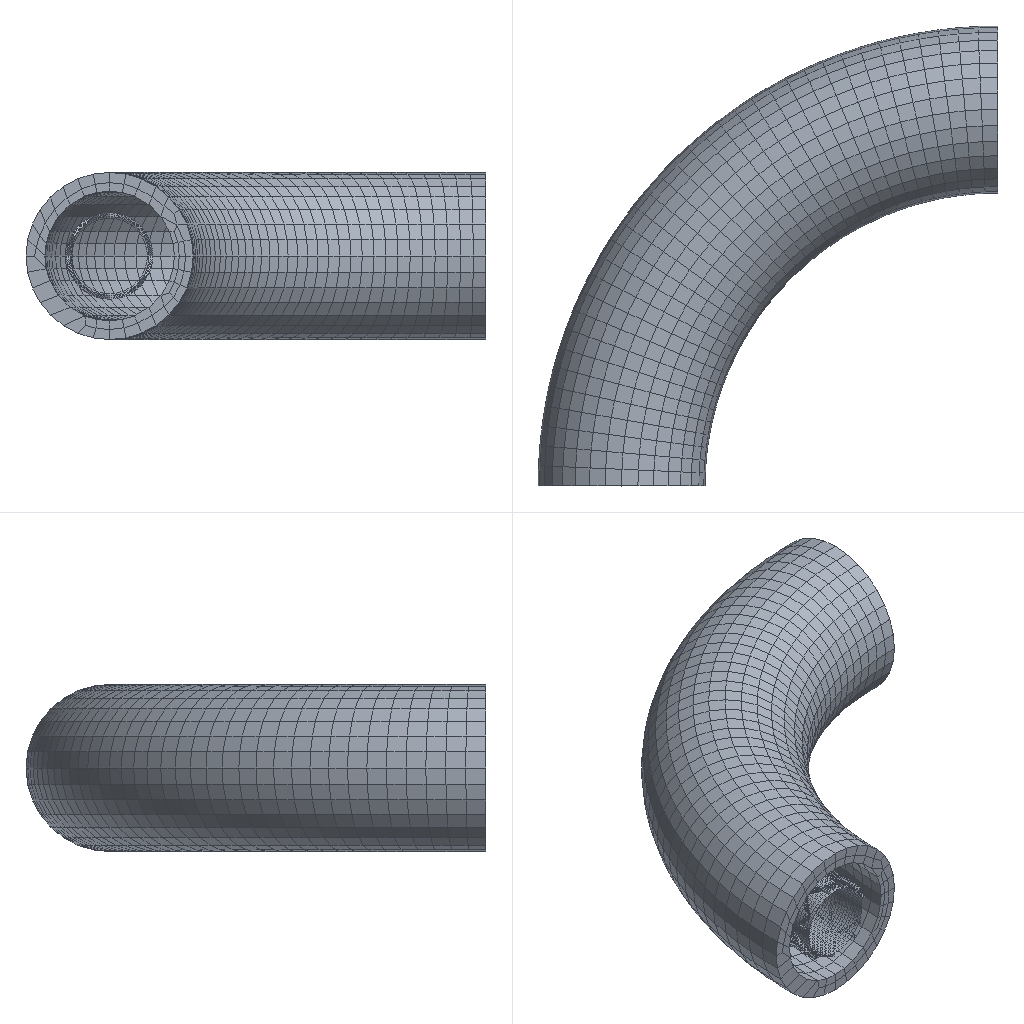Simulation study | abaqus
Set-up summary:
category,name,step,type,value,unit,region
solver,abaqus
solver,version,,,Abaqus/Explicit 2020
units,not stated in the deck,,not stated
analysis,deck,,transient,transient
load_step,Step-1,Step-1,transient
load_step,requested,,,1
mesh,nodes,,,9006
mesh,elements,,,15441
element_type,S4R,,shell,1134
element_type,C3D4H,,solid,12039
element_type,C3D8R,,solid,2268
load,load commands in deck,,count,1
bc,support commands in deck,,count,3
material,SHELL-BALLOON,,in results
material,SS316LN,,in results
material,OGDEN ARTERIAL VESSEL,,in results
check,setup vs results,,match,"per instance, exact: element labels, types and connectivity; labels of the nodes the elements use; coordinates of those nodes at SINGLE_PRECISION in 3 of 3 instance(s)"
Abaqus input file, long lists of numbers shortened:
*Heading
** Job name: Job-2 Model name: Model-1-Copy
** Generated by: Abaqus/CAE 2020
*Preprint, echo=NO, model=NO, history=NO, contact=NO
**
** PARTS
**
*Part, name=P05vessel-r10-220518
*Node
      1,  -12.22,           0., -2.5200424e-09
      2,  -12.177,           0.,  0.4331
** (3439 more lines like these left out)
*Element, type=C3D8R
   1,   68,   66,    1,    2,  161,  159,   94,   95
   2,   34,   66,   68,   33,  127,  159,  161,  126
** (2266 more lines like these left out)
*Nset, nset=Set-1, generate
    1,  3441,     1
*Elset, elset=Set-1, generate
    1,  2268,     1
** Section: Section-2
*Solid Section, elset=Set-1, material="ogden arterial vessel"
,
*End Part
**
*Part, name=Part-1
*Node
      1,  0.995,  0.9, -0.09957
      2,  0.9802,  0.9,  -0.1981
** (1195 more lines like these left out)
*Element, type=S4R
   1,   63,    1,   64,  126
   2,    1,    2,   65,   64
** (1132 more lines like these left out)
*Nset, nset=Set-1, generate
    1,  1197,     1
*Elset, elset=Set-1, generate
    1,  1134,     1
*Nset, nset=Set-3, generate
    1,  1197,     1
*Elset, elset=Set-3, generate
    1,  1134,     1
** Section: Section-1
*Shell Section, elset=Set-1, material=shell-balloon
1., 5
*End Part
**
*Part, name=wrap3layers-R10-220518
*Node
      1, -0.523,  0.55, -0.9058
      2, -0.2032,  0.2828,  -1.026
** (4366 more lines like these left out)
*Element, type=C3D4H
    1, 3584, 3585, 3569, 1457
    2, 3584, 3586,  188, 2546
** (12037 more lines like these left out)
*Nset, nset=Set-1, generate
    1,  4368,     1
*Elset, elset=Set-1, generate
     1,  12039,      1
*Nset, nset=Set-6, generate
    1,  4368,     1
*Elset, elset=Set-6, generate
     1,  12039,      1
** Section: Section-3
*Solid Section, elset=Set-1, material=SS316LN
,
*End Part
**
**
** ASSEMBLY
**
*Assembly, name=Assembly
**
*Instance, name=P05vessel-r10-220518-1, part=P05vessel-r10-220518
   10.11,         -0.9,    -0.284
*End Instance
**
*Instance, name=Part-1-1, part=Part-1
    0.1102,           0.,    -0.284
*End Instance
**
*Instance, name=wrap3layers-R10-220518-1, part=wrap3layers-R10-220518
    0.1102,         -0.9,    -0.284
*End Instance
**
*Nset, nset=Set-1, instance=P05vessel-r10-220518-1, generate
 3349,  3441,     1
*Elset, elset=Set-1, instance=P05vessel-r10-220518-1, generate
 2206,  2268,     1
*Nset, nset=Set-2, instance=Part-1-1, generate
 1135,  1197,     1
*Elset, elset=Set-2, instance=Part-1-1, generate
 1072,  1134,     1
*Nset, nset=Set-3, instance=P05vessel-r10-220518-1, generate
 3349,  3441,     1
*Elset, elset=Set-3, instance=P05vessel-r10-220518-1, generate
 2206,  2268,     1
*Nset, nset=Set-4, instance=Part-1-1, generate
 1135,  1197,     1
*Elset, elset=Set-4, instance=Part-1-1, generate
 1072,  1134,     1
*Nset, nset=Set-5, instance=wrap3layers-R10-220518-1
  135,  136,  137,  138, 1179, 1185
*Elset, elset=Set-5, instance=wrap3layers-R10-220518-1
  2910,  2912, 10089, 10115
*Nset, nset=Set-6, instance=P05vessel-r10-220518-1, generate
  1,  93,   1
*Elset, elset=Set-6, instance=P05vessel-r10-220518-1, generate
  1,  63,   1
*Nset, nset=Set-7, instance=P05vessel-r10-220518-1, generate
  1,  93,   1
*Nset, nset=Set-7, instance=Part-1-1, generate
 1135,  1197,     1
*Elset, elset=Set-7, instance=P05vessel-r10-220518-1, generate
  1,  63,   1
*Elset, elset=Set-7, instance=Part-1-1, generate
 1072,  1134,     1
*Nset, nset=Set-8, instance=P05vessel-r10-220518-1, generate
  1,  93,   1
*Elset, elset=Set-8, instance=P05vessel-r10-220518-1, generate
  1,  63,   1
*Nset, nset=Set-9, instance=Part-1-1, generate
 1135,  1197,     1
*Elset, elset=Set-9, instance=Part-1-1, generate
 1072,  1134,     1
*Nset, nset=Set-10, instance=wrap3layers-R10-220518-1
  135,  136,  137,  138,  147,  148,  149,  150,  159,  160,  161,  162,  287,  288,  289,  290
  299,  300,  301,  302, 1179, 1185, 1244, 1249, 1305, 1309, 2129, 2133, 2192, 2197
*Elset, elset=Set-10, instance=wrap3layers-R10-220518-1
   937,  2442,  2548,  2807,  2910,  2912,  2915,  2916,  4317,  4613,  4618,  4622,  4624,  9087,  9090,  9126
  9561,  9600, 10089, 10115
*Elset, elset=_Surf-7_SPOS, internal, instance=Part-1-1, generate
    1,  1134,     1
*Surface, type=ELEMENT, name=Surf-7
_Surf-7_SPOS, SPOS
*Elset, elset=_Surf-8_SPOS, internal, instance=Part-1-1, generate
    1,  1134,     1
*Surface, type=ELEMENT, name=Surf-8
_Surf-8_SPOS, SPOS
*Elset, elset=_Surf-15_SPOS, internal, instance=Part-1-1, generate
    1,  1134,     1
*Surface, type=ELEMENT, name=Surf-15
_Surf-15_SPOS, SPOS
*Elset, elset=_m_Surf-1_SNEG, internal, instance=Part-1-1, generate
    1,  1134,     1
*Surface, type=ELEMENT, name=m_Surf-1
_m_Surf-1_SNEG, SNEG
*Elset, elset=_m_Surf-3_S3, internal, instance=wrap3layers-R10-220518-1
    50,    60,    77,   128,   131,   135,   347,   433,   439,   440,   470,   475,   486,   493,   502,   539
   718,   754,   759,   775,   972,   979,  1011,  1036,  1055,  1083,  1146,  1174,  1237,  1257,  1259,  1315
** (23 more lines like these left out)
*Elset, elset=_m_Surf-3_S1, internal, instance=wrap3layers-R10-220518-1
   284,  5570,  5738,  6653,  7904,  8010,  8072,  8078,  8127,  8131,  8229,  8243,  8525,  8528,  8577,  8584
  8589,  8590,  8594,  8686,  8801,  9018,  9062,  9678,  9724,  9747,  9774,  9791,  9890, 10009, 10609, 10626
** (1 more lines like these left out)
*Elset, elset=_m_Surf-3_S2, internal, instance=wrap3layers-R10-220518-1
  5035,  5699,  5848,  6144,  6166,  6635,  6637,  6676,  6775,  7137,  7143,  7630,  7856,  8003,  8027,  8079
  8312,  8323,  8374,  8539,  8569,  8587,  8682,  8785,  8803,  8981,  8995,  9064,  9143,  9195,  9200,  9247
** (3 more lines like these left out)
*Elset, elset=_m_Surf-3_S4, internal, instance=wrap3layers-R10-220518-1
  5723,  6031,  6055,  6210,  6217,  6370,  6627,  6659,  6682,  7078,  7167,  7181,  7324,  7532,  7582,  7647
  7669,  7969,  8069,  8073,  8088,  8123,  8258,  8298,  8317,  8322,  8330,  8358,  8526,  8601,  8667,  8672
** (5 more lines like these left out)
*Surface, type=ELEMENT, name=m_Surf-3
_m_Surf-3_S3, S3
_m_Surf-3_S1, S1
_m_Surf-3_S2, S2
_m_Surf-3_S4, S4
*Elset, elset=_m_Surf-5_S3, internal, instance=wrap3layers-R10-220518-1
     5,    50,    60,    69,    77,    91,    95,   108,   110,   115,   128,   131,   135,   144,   169,   207
   213,   329,   347,   372,   415,   433,   439,   440,   450,   453,   470,   475,   486,   493,   502,   539
** (49 more lines like these left out)
*Elset, elset=_m_Surf-5_S1, internal, instance=wrap3layers-R10-220518-1
   174,   284,  1690,  3280,  3431,  3438,  3617,  3763,  3976,  3978,  3998,  4007,  4254,  4260,  4271,  4445
  4488,  4647,  4697,  4716,  4773,  4794,  4946,  5128,  5158,  5174,  5238,  5440,  5570,  5595,  5643,  5730
** (4 more lines like these left out)
*Elset, elset=_m_Surf-5_S4, internal, instance=wrap3layers-R10-220518-1
  2001,  3180,  3188,  3224,  3281,  3306,  3631,  3654,  3667,  3755,  3758,  3762,  3766,  3799,  3975,  3987
  3991,  4045,  4231,  4239,  4255,  4264,  4265,  4279,  4282,  4349,  4359,  4362,  4444,  4592,  4638,  4742
** (11 more lines like these left out)
*Elset, elset=_m_Surf-5_S2, internal, instance=wrap3layers-R10-220518-1
  3194,  3651,  3973,  4000,  4038,  4046,  4094,  4138,  4448,  4704,  4728,  4729,  4764,  4784,  4878,  5035
  5093,  5112,  5124,  5143,  5150,  5222,  5229,  5234,  5252,  5334,  5359,  5504,  5556,  5699,  5784,  5785
** (7 more lines like these left out)
*Surface, type=ELEMENT, name=m_Surf-5
_m_Surf-5_S3, S3
_m_Surf-5_S1, S1
_m_Surf-5_S4, S4
_m_Surf-5_S2, S2
*Elset, elset=_m_Surf-9_SNEG, internal, instance=Part-1-1, generate
    1,  1134,     1
*Surface, type=ELEMENT, name=m_Surf-9
_m_Surf-9_SNEG, SNEG
*Elset, elset=_m_Surf-11_SNEG, internal, instance=Part-1-1, generate
    1,  1134,     1
*Surface, type=ELEMENT, name=m_Surf-11
_m_Surf-11_SNEG, SNEG
*Elset, elset=_m_Surf-13_S3, internal, instance=wrap3layers-R10-220518-1
     5,    50,    60,    69,    77,    91,    95,   108,   110,   115,   128,   131,   135,   144,   169,   207
   213,   329,   347,   372,   415,   433,   439,   440,   450,   453,   470,   475,   486,   493,   502,   539
** (49 more lines like these left out)
*Elset, elset=_m_Surf-13_S1, internal, instance=wrap3layers-R10-220518-1
   174,   284,  1690,  3280,  3431,  3438,  3617,  3763,  3976,  3978,  3998,  4007,  4254,  4260,  4271,  4445
  4488,  4647,  4697,  4716,  4773,  4794,  4946,  5128,  5158,  5174,  5238,  5440,  5570,  5595,  5643,  5730
** (4 more lines like these left out)
*Elset, elset=_m_Surf-13_S4, internal, instance=wrap3layers-R10-220518-1
  2001,  3180,  3188,  3224,  3281,  3306,  3631,  3654,  3667,  3755,  3758,  3762,  3766,  3799,  3975,  3987
  3991,  4045,  4231,  4239,  4255,  4264,  4265,  4279,  4282,  4349,  4359,  4362,  4444,  4592,  4638,  4742
** (11 more lines like these left out)
*Elset, elset=_m_Surf-13_S2, internal, instance=wrap3layers-R10-220518-1
  3194,  3651,  3973,  4000,  4038,  4046,  4094,  4138,  4448,  4704,  4728,  4729,  4764,  4784,  4878,  5035
  5093,  5112,  5124,  5143,  5150,  5222,  5229,  5234,  5252,  5334,  5359,  5504,  5556,  5699,  5784,  5785
** (7 more lines like these left out)
*Surface, type=ELEMENT, name=m_Surf-13
_m_Surf-13_S3, S3
_m_Surf-13_S1, S1
_m_Surf-13_S4, S4
_m_Surf-13_S2, S2
*Elset, elset=_m_Surf-16_S4, internal, instance=P05vessel-r10-220518-1
    5,   17,   22,   32,   39,   53,   61,   62,   68,   80,   85,   95,  102,  116,  124,  125
  131,  143,  148,  158,  165,  179,  187,  188,  194,  206,  211,  221,  228,  242,  250,  251
** (16 more lines like these left out)
*Elset, elset=_m_Surf-16_S3, internal, instance=P05vessel-r10-220518-1
    8,   27,   38,   41,   44,   71,   90,  101,  104,  107,  134,  153,  164,  167,  170,  197
  216,  227,  230,  233,  260,  279,  290,  293,  296,  323,  342,  353,  356,  359,  386,  405
** (10 more lines like these left out)
*Elset, elset=_m_Surf-16_S5, internal, instance=P05vessel-r10-220518-1
    9,   28,   37,   43,   45,   46,   47,   58,   60,   72,   91,  100,  106,  108,  109,  110
  121,  123,  135,  154,  163,  169,  171,  172,  173,  184,  186,  198,  217,  226,  232,  234
** (19 more lines like these left out)
*Elset, elset=_m_Surf-16_S6, internal, instance=P05vessel-r10-220518-1
    2,    3,    4,    6,   13,   36,   65,   66,   67,   69,   76,   99,  128,  129,  130,  132
  139,  162,  191,  192,  193,  195,  202,  225,  254,  255,  256,  258,  265,  288,  317,  318
** (12 more lines like these left out)
*Surface, type=ELEMENT, name=m_Surf-16
_m_Surf-16_S4, S4
_m_Surf-16_S3, S3
_m_Surf-16_S6, S6
_m_Surf-16_S5, S5
*Elset, elset=_s_Surf-1_S3, internal, instance=wrap3layers-R10-220518-1
    18,    67,   109,   149,   179,   199,   230,   278,   286,   288,   291,   292,   309,   310,   335,   365
   369,   384,   411,   457,   498,   510,   532,   547,   551,   552,   577,   585,   613,   675,   702,   737
** (54 more lines like these left out)
*Elset, elset=_s_Surf-1_S1, internal, instance=wrap3layers-R10-220518-1
   154,   220,  3101,  3247,  3256,  3276,  3342,  3573,  3671,  3682,  3760,  4061,  4148,  4272,  4392,  4567
  4753,  5162,  5251,  5559,  5874,  5899,  5952,  6123,  6169,  6255,  6491,  6629,  6922,  7002,  7090,  7142
** (2 more lines like these left out)
*Elset, elset=_s_Surf-1_S4, internal, instance=wrap3layers-R10-220518-1
   258,  3048,  3221,  3298,  3301,  3302,  3310,  3320,  3455,  3461,  3499,  3738,  3741,  3747,  3751,  3783
  3802,  4068,  4091,  4243,  4256,  4401,  4545,  4569,  4677,  4909,  4948,  5137,  5191,  5198,  5213,  5444
** (7 more lines like these left out)
*Elset, elset=_s_Surf-1_S2, internal, instance=wrap3layers-R10-220518-1
    58,   308,  2870,  3178,  3229,  3232,  3239,  3442,  3520,  3670,  3773,  3813,  3911,  3957,  4002,  4050
  4228,  4287,  4337,  4384,  4394,  4420,  4588,  4663,  4700,  4774,  4818,  4903,  5087,  5183,  5256,  5304
** (7 more lines like these left out)
*Surface, type=ELEMENT, name=s_Surf-1
_s_Surf-1_S3, S3
_s_Surf-1_S1, S1
_s_Surf-1_S4, S4
_s_Surf-1_S2, S2
*Elset, elset=_s_Surf-3_S6, internal, instance=P05vessel-r10-220518-1
    2,    3,    4,    6,   13,   65,   66,   67,   69,   76,  128,  129,  130,  132,  139,  191
  192,  193,  195,  202,  254,  255,  256,  258,  265,  317,  318,  319,  321,  328,  380,  381
** (10 more lines like these left out)
*Elset, elset=_s_Surf-3_S4, internal, instance=P05vessel-r10-220518-1
    5,   17,   62,   68,   80,  125,  131,  143,  188,  194,  206,  251,  257,  269,  314,  320
  332,  377,  383,  395,  440,  446,  458,  503,  509,  521,  566,  572,  584,  629,  635,  647
** (5 more lines like these left out)
*Elset, elset=_s_Surf-3_S3, internal, instance=P05vessel-r10-220518-1
    8,   41,   44,   71,  104,  107,  134,  167,  170,  197,  230,  233,  260,  293,  296,  323
  356,  359,  386,  419,  422,  449,  482,  485,  512,  545,  548,  575,  608,  611,  638,  671
** (5 more lines like these left out)
*Elset, elset=_s_Surf-3_S5, internal, instance=P05vessel-r10-220518-1
    9,   43,   47,   72,  106,  110,  135,  169,  173,  198,  232,  236,  261,  295,  299,  324
  358,  362,  387,  421,  425,  450,  484,  488,  513,  547,  551,  576,  610,  614,  639,  673
** (5 more lines like these left out)
*Surface, type=ELEMENT, name=s_Surf-3
_s_Surf-3_S6, S6
_s_Surf-3_S4, S4
_s_Surf-3_S3, S3
_s_Surf-3_S5, S5
*Elset, elset=_s_Surf-5_S4, internal, instance=P05vessel-r10-220518-1
    5,   17,   22,   32,   39,   53,   61,   62,   68,   80,   85,   95,  102,  116,  124,  125
  131,  143,  148,  158,  165,  179,  187,  188,  194,  206,  211,  221,  228,  242,  250,  251
** (16 more lines like these left out)
*Elset, elset=_s_Surf-5_S3, internal, instance=P05vessel-r10-220518-1
    8,   27,   38,   41,   44,   71,   90,  101,  104,  107,  134,  153,  164,  167,  170,  197
  216,  227,  230,  233,  260,  279,  290,  293,  296,  323,  342,  353,  356,  359,  386,  405
** (10 more lines like these left out)
*Elset, elset=_s_Surf-5_S5, internal, instance=P05vessel-r10-220518-1
    9,   28,   37,   43,   45,   46,   47,   58,   60,   72,   91,  100,  106,  108,  109,  110
  121,  123,  135,  154,  163,  169,  171,  172,  173,  184,  186,  198,  217,  226,  232,  234
** (19 more lines like these left out)
*Elset, elset=_s_Surf-5_S6, internal, instance=P05vessel-r10-220518-1
    2,    3,    4,    6,   13,   36,   65,   66,   67,   69,   76,   99,  128,  129,  130,  132
  139,  162,  191,  192,  193,  195,  202,  225,  254,  255,  256,  258,  265,  288,  317,  318
** (12 more lines like these left out)
*Surface, type=ELEMENT, name=s_Surf-5
_s_Surf-5_S4, S4
_s_Surf-5_S3, S3
_s_Surf-5_S6, S6
_s_Surf-5_S5, S5
*Elset, elset=_s_Surf-9_S3, internal, instance=wrap3layers-R10-220518-1
    18,    67,   109,   149,   179,   199,   230,   278,   286,   288,   291,   292,   309,   310,   335,   365
   369,   384,   411,   457,   498,   510,   532,   547,   551,   552,   577,   585,   613,   675,   702,   737
** (54 more lines like these left out)
*Elset, elset=_s_Surf-9_S1, internal, instance=wrap3layers-R10-220518-1
   154,   220,  3101,  3247,  3256,  3276,  3342,  3573,  3671,  3682,  3760,  4061,  4148,  4272,  4392,  4567
  4753,  5162,  5251,  5559,  5874,  5899,  5952,  6123,  6169,  6255,  6491,  6629,  6922,  7002,  7090,  7142
** (2 more lines like these left out)
*Elset, elset=_s_Surf-9_S4, internal, instance=wrap3layers-R10-220518-1
   258,  3048,  3221,  3298,  3301,  3302,  3310,  3320,  3455,  3461,  3499,  3738,  3741,  3747,  3751,  3783
  3802,  4068,  4091,  4243,  4256,  4401,  4545,  4569,  4677,  4909,  4948,  5137,  5191,  5198,  5213,  5444
** (7 more lines like these left out)
*Elset, elset=_s_Surf-9_S2, internal, instance=wrap3layers-R10-220518-1
    58,   308,  2870,  3178,  3229,  3232,  3239,  3442,  3520,  3670,  3773,  3813,  3911,  3957,  4002,  4050
  4228,  4287,  4337,  4384,  4394,  4420,  4588,  4663,  4700,  4774,  4818,  4903,  5087,  5183,  5256,  5304
** (7 more lines like these left out)
*Surface, type=ELEMENT, name=s_Surf-9
_s_Surf-9_S3, S3
_s_Surf-9_S1, S1
_s_Surf-9_S4, S4
_s_Surf-9_S2, S2
*Elset, elset=_s_Surf-11_S3, internal, instance=wrap3layers-R10-220518-1
    18,    67,   109,   149,   179,   199,   230,   278,   286,   288,   291,   292,   309,   310,   335,   365
   369,   384,   411,   457,   498,   510,   532,   547,   551,   552,   577,   585,   613,   675,   702,   737
** (54 more lines like these left out)
*Elset, elset=_s_Surf-11_S1, internal, instance=wrap3layers-R10-220518-1
   154,   220,  3101,  3247,  3256,  3276,  3342,  3573,  3671,  3682,  3760,  4061,  4148,  4272,  4392,  4567
  4753,  5162,  5251,  5559,  5874,  5899,  5952,  6123,  6169,  6255,  6491,  6629,  6922,  7002,  7090,  7142
** (2 more lines like these left out)
*Elset, elset=_s_Surf-11_S4, internal, instance=wrap3layers-R10-220518-1
   258,  3048,  3221,  3298,  3301,  3302,  3310,  3320,  3455,  3461,  3499,  3738,  3741,  3747,  3751,  3783
  3802,  4068,  4091,  4243,  4256,  4401,  4545,  4569,  4677,  4909,  4948,  5137,  5191,  5198,  5213,  5444
** (7 more lines like these left out)
*Elset, elset=_s_Surf-11_S2, internal, instance=wrap3layers-R10-220518-1
    58,   308,  2870,  3178,  3229,  3232,  3239,  3442,  3520,  3670,  3773,  3813,  3911,  3957,  4002,  4050
  4228,  4287,  4337,  4384,  4394,  4420,  4588,  4663,  4700,  4774,  4818,  4903,  5087,  5183,  5256,  5304
** (7 more lines like these left out)
*Surface, type=ELEMENT, name=s_Surf-11
_s_Surf-11_S3, S3
_s_Surf-11_S1, S1
_s_Surf-11_S4, S4
_s_Surf-11_S2, S2
*Elset, elset=_s_Surf-13_S4, internal, instance=P05vessel-r10-220518-1
    5,   17,   22,   32,   39,   53,   61,   62,   68,   80,   85,   95,  102,  116,  124,  125
  131,  143,  148,  158,  165,  179,  187,  188,  194,  206,  211,  221,  228,  242,  250,  251
** (16 more lines like these left out)
*Elset, elset=_s_Surf-13_S3, internal, instance=P05vessel-r10-220518-1
    8,   27,   38,   41,   44,   71,   90,  101,  104,  107,  134,  153,  164,  167,  170,  197
  216,  227,  230,  233,  260,  279,  290,  293,  296,  323,  342,  353,  356,  359,  386,  405
** (10 more lines like these left out)
*Elset, elset=_s_Surf-13_S5, internal, instance=P05vessel-r10-220518-1
    9,   28,   37,   43,   45,   46,   47,   58,   60,   72,   91,  100,  106,  108,  109,  110
  121,  123,  135,  154,  163,  169,  171,  172,  173,  184,  186,  198,  217,  226,  232,  234
** (19 more lines like these left out)
*Elset, elset=_s_Surf-13_S6, internal, instance=P05vessel-r10-220518-1
    2,    3,    4,    6,   13,   36,   65,   66,   67,   69,   76,   99,  128,  129,  130,  132
  139,  162,  191,  192,  193,  195,  202,  225,  254,  255,  256,  258,  265,  288,  317,  318
** (12 more lines like these left out)
*Surface, type=ELEMENT, name=s_Surf-13
_s_Surf-13_S4, S4
_s_Surf-13_S3, S3
_s_Surf-13_S6, S6
_s_Surf-13_S5, S5
*Elset, elset=_s_Surf-16_S2, internal, instance=wrap3layers-R10-220518-1
    58,   111,   259,   284,   298,   308,   309,   555,   620,   632,   722,   760,   801,   959,  1072,  1466
  1657,  1672,  1786,  1911,  2354,  2461,  2612,  2642,  2870,  2948,  2994,  3060,  3136,  3178,  3184,  3194
** (49 more lines like these left out)
*Elset, elset=_s_Surf-16_S3, internal, instance=wrap3layers-R10-220518-1
     3,     5,    17,    18,    23,    24,    32,    35,    37,    40,    46,    48,    50,    60,    66,    67
    69,    74,    77,    80,    87,    91,    92,    95,    98,   102,   108,   109,   110,   114,   115,   121
** (311 more lines like these left out)
*Elset, elset=_s_Surf-16_S4, internal, instance=wrap3layers-R10-220518-1
   174,   258,   827,  1414,  1670,  1681,  1690,  1985,  2001,  2312,  3048,  3091,  3166,  3180,  3188,  3189
  3191,  3192,  3194,  3221,  3224,  3225,  3237,  3238,  3280,  3281,  3282,  3298,  3300,  3301,  3302,  3304
** (49 more lines like these left out)
*Elset, elset=_s_Surf-16_S1, internal, instance=wrap3layers-R10-220518-1
    63,   154,   174,   220,   258,   284,   385,   690,  1506,  1690,  1918,  1987,  2317,  3088,  3101,  3178
  3180,  3181,  3188,  3227,  3243,  3247,  3252,  3255,  3256,  3259,  3261,  3262,  3263,  3275,  3276,  3280
** (35 more lines like these left out)
*Surface, type=ELEMENT, name=s_Surf-16
_s_Surf-16_S2, S2
_s_Surf-16_S3, S3
_s_Surf-16_S4, S4
_s_Surf-16_S1, S1
*Elset, elset=_s_Surf-18_SNEG, internal, instance=Part-1-1, generate
    1,  1134,     1
*Surface, type=ELEMENT, name=s_Surf-18
_s_Surf-18_SNEG, SNEG
*End Assembly
*Amplitude, name=Amp-1
             0.,              0.,           0.008,              1.,            0.01,              0.
**
** MATERIALS
**
*Material, name=SS316LN
*Density
 7.99e-09,
*Elastic
196000., 0.3
*Plastic
205.,    0.
515., 0.599
*Material, name="ogden arterial vessel"
*Density
 1.07e-09,
*Hyperelastic, n=3, ogden
 -4.73,    -0.39,      1.7,     4.41,     3.09,    -3.25, 3.63e-06,       0.
       0.,
*Material, name=shell-balloon
*Density
 1.07e-09,
*Elastic
 25.8, 0.32
**
** INTERACTION PROPERTIES
**
*Surface Interaction, name=IntProp-1
*Friction
 0.15,
*Surface Behavior, pressure-overclosure=HARD
** ----------------------------------------------------------------
**
** STEP: Step-1
**
*Step, name=Step-1, nlgeom=YES
*Dynamic, Explicit
, 0.01
*Bulk Viscosity
0.06, 1.2
** Mass Scaling: Semi-Automatic
**               Whole Model
*Fixed Mass Scaling, factor=5000.
**
** BOUNDARY CONDITIONS
**
** Name: BC-1 Type: 对称/反对称/完全固定
*Boundary
Set-3, ENCASTRE
** Name: BC-3 Type: 对称/反对称/完全固定
*Boundary
Set-8, YSYMM
** Name: BC-5 Type: 对称/反对称/完全固定
*Boundary
Set-10, YSYMM
**
** LOADS
**
** Name: Load-1   Type: Pressure
*Dsload, amplitude=Amp-1
Surf-15, P, 10.
**
** INTERACTIONS
**
** Interaction: Int-3
*Contact, op=NEW
*Contact Inclusions, ALL EXTERIOR
*Contact Property Assignment
 ,  , IntProp-1
**
** OUTPUT REQUESTS
**
*Restart, write, number interval=1, time marks=NO
**
** FIELD OUTPUT: F-Output-1
**
*Output, field, number interval=100
*Node Output
A, CF, RF, U, V
*Element Output, directions=YES
E, LE, MISES, MISESMAX, PE, PEEQ, PEMAG, S, SSAVG
*Contact Output
CDISP, CSTRESS
**
** HISTORY OUTPUT: H-Output-1
**
*Output, history, variable=PRESELECT
*End Step
Results summary:
result,step,Step-1,completed,increments=78857 time=0.01/0.01
result,analysis,,,transient
result,last_loadstep,,,1
result,primary field,,,"U, UR"
result,reaction total,,FX,-0.1031,model units
result,reaction total,,FY,-4.552,model units
result,reaction total,,FZ,-4e-06,model units